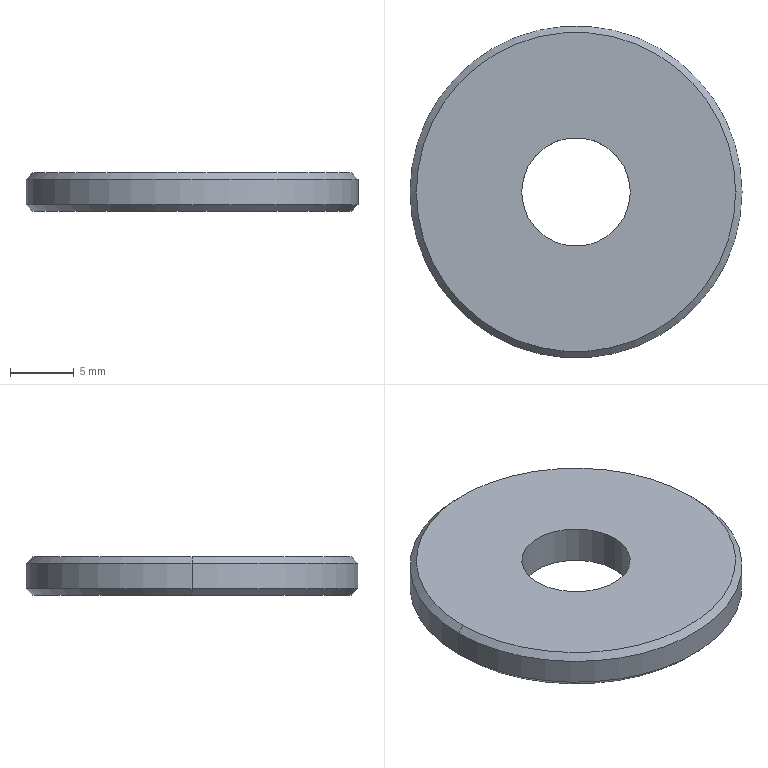Part | STEP file | 11-FG-SJ01711 | 1 solid | 10 faces | box 26 x 26 x 3 mm | volume 1402 mm3 | cone 4 | cylinder 4 | plane 2 | commonest cylinder face diameters 8.5 x2 26 x2
STEP:
#1=CARTESIAN_POINT('',(12.5,0.,3.));
#2=VERTEX_POINT('',#1);
#3=CARTESIAN_POINT('',(-12.5,0.,3.));
#4=VERTEX_POINT('',#3);
#5=CARTESIAN_POINT('',(0.,0.,3.));
#6=DIRECTION('',(0.,0.,1.));
#7=DIRECTION('',(1.,0.,0.));
#8=AXIS2_PLACEMENT_3D('',#5,#6,#7);
#9=CIRCLE('',#8,12.5);
#10=EDGE_CURVE('',#2,#4,#9,.T.);
#11=ORIENTED_EDGE('',*,*,#10,.F.);
#12=CARTESIAN_POINT('',(13.,0.,2.5));
#13=VERTEX_POINT('',#12);
#14=CARTESIAN_POINT('',(12.5,0.,3.));
#15=DIRECTION('',(0.7071,0.,-0.7071));
#16=VECTOR('',#15,1000.);
#17=LINE('',#14,#16);
#18=EDGE_CURVE('',#2,#13,#17,.T.);
#19=ORIENTED_EDGE('',*,*,#18,.T.);
#20=CARTESIAN_POINT('',(-13.,0.,2.5));
#21=VERTEX_POINT('',#20);
#22=CARTESIAN_POINT('',(0.,0.,2.5));
#23=DIRECTION('',(0.,0.,-1.));
#24=DIRECTION('',(1.,0.,0.));
#25=AXIS2_PLACEMENT_3D('',#22,#23,#24);
#26=CIRCLE('',#25,13.);
#27=EDGE_CURVE('',#21,#13,#26,.T.);
#28=ORIENTED_EDGE('',*,*,#27,.F.);
#29=CARTESIAN_POINT('',(-12.5,0.,3.));
#30=DIRECTION('',(-0.7071,0.,-0.7071));
#31=VECTOR('',#30,1000.);
#32=LINE('',#29,#31);
#33=EDGE_CURVE('',#4,#21,#32,.T.);
#34=ORIENTED_EDGE('',*,*,#33,.F.);
#35=EDGE_LOOP('',(#11,#19,#28,#34));
#36=FACE_OUTER_BOUND('',#35,.T.);
#37=CARTESIAN_POINT('',(0.,0.,3.));
#38=DIRECTION('',(0.,0.,-1.));
#39=DIRECTION('',(-1.,0.,0.));
#40=AXIS2_PLACEMENT_3D('',#37,#38,#39);
#41=CONICAL_SURFACE('',#40,12.5,0.7854);
#42=ADVANCED_FACE('',(#36),#41,.T.);
#43=CARTESIAN_POINT('',(-12.5,0.,0.));
#44=VERTEX_POINT('',#43);
#45=CARTESIAN_POINT('',(12.5,0.,0.));
#46=VERTEX_POINT('',#45);
#47=CARTESIAN_POINT('',(0.,0.,0.));
#48=DIRECTION('',(0.,0.,-1.));
#49=DIRECTION('',(1.,0.,0.));
#50=AXIS2_PLACEMENT_3D('',#47,#48,#49);
#51=CIRCLE('',#50,12.5);
#52=EDGE_CURVE('',#44,#46,#51,.T.);
#53=ORIENTED_EDGE('',*,*,#52,.F.);
#54=CARTESIAN_POINT('',(-13.,0.,0.5));
#55=VERTEX_POINT('',#54);
#56=CARTESIAN_POINT('',(-13.,0.,0.5));
#57=DIRECTION('',(-0.7071,0.,0.7071));
#58=VECTOR('',#57,1000.);
#59=LINE('',#56,#58);
#60=EDGE_CURVE('',#44,#55,#59,.T.);
#61=ORIENTED_EDGE('',*,*,#60,.T.);
#62=CARTESIAN_POINT('',(13.,0.,0.5));
#63=VERTEX_POINT('',#62);
#64=CARTESIAN_POINT('',(0.,0.,0.5));
#65=DIRECTION('',(0.,0.,1.));
#66=DIRECTION('',(1.,0.,0.));
#67=AXIS2_PLACEMENT_3D('',#64,#65,#66);
#68=CIRCLE('',#67,13.);
#69=EDGE_CURVE('',#63,#55,#68,.T.);
#70=ORIENTED_EDGE('',*,*,#69,.F.);
#71=CARTESIAN_POINT('',(13.,0.,0.5));
#72=DIRECTION('',(0.7071,0.,0.7071));
#73=VECTOR('',#72,1000.);
#74=LINE('',#71,#73);
#75=EDGE_CURVE('',#46,#63,#74,.T.);
#76=ORIENTED_EDGE('',*,*,#75,.F.);
#77=EDGE_LOOP('',(#53,#61,#70,#76));
#78=FACE_OUTER_BOUND('',#77,.T.);
#79=CARTESIAN_POINT('',(0.,0.,0.5));
#80=DIRECTION('',(0.,0.,1.));
#81=DIRECTION('',(1.,0.,0.));
#82=AXIS2_PLACEMENT_3D('',#79,#80,#81);
#83=CONICAL_SURFACE('',#82,13.,0.7854);
#84=ADVANCED_FACE('',(#78),#83,.T.);
#85=CARTESIAN_POINT('',(-4.25,0.,3.));
#86=VERTEX_POINT('',#85);
#87=CARTESIAN_POINT('',(4.25,0.,3.));
#88=VERTEX_POINT('',#87);
#89=CARTESIAN_POINT('',(0.,0.,3.));
#90=DIRECTION('',(0.,0.,1.));
#91=DIRECTION('',(1.,0.,0.));
#92=AXIS2_PLACEMENT_3D('',#89,#90,#91);
#93=CIRCLE('',#92,4.25);
#94=EDGE_CURVE('',#86,#88,#93,.T.);
#95=ORIENTED_EDGE('',*,*,#94,.T.);
#96=CARTESIAN_POINT('',(4.25,0.,0.));
#97=VERTEX_POINT('',#96);
#98=CARTESIAN_POINT('',(4.25,0.,3.));
#99=DIRECTION('',(0.,0.,-1.));
#100=VECTOR('',#99,1000.);
#101=LINE('',#98,#100);
#102=EDGE_CURVE('',#88,#97,#101,.T.);
#103=ORIENTED_EDGE('',*,*,#102,.T.);
#104=CARTESIAN_POINT('',(-4.25,0.,0.));
#105=VERTEX_POINT('',#104);
#106=CARTESIAN_POINT('',(0.,0.,0.));
#107=DIRECTION('',(0.,0.,1.));
#108=DIRECTION('',(1.,0.,0.));
#109=AXIS2_PLACEMENT_3D('',#106,#107,#108);
#110=CIRCLE('',#109,4.25);
#111=EDGE_CURVE('',#105,#97,#110,.T.);
#112=ORIENTED_EDGE('',*,*,#111,.F.);
#113=CARTESIAN_POINT('',(-4.25,0.,3.));
#114=DIRECTION('',(0.,0.,-1.));
#115=VECTOR('',#114,1000.);
#116=LINE('',#113,#115);
#117=EDGE_CURVE('',#86,#105,#116,.T.);
#118=ORIENTED_EDGE('',*,*,#117,.F.);
#119=EDGE_LOOP('',(#95,#103,#112,#118));
#120=FACE_OUTER_BOUND('',#119,.T.);
#121=CARTESIAN_POINT('',(0.,0.,3.));
#122=DIRECTION('',(0.,0.,-1.));
#123=DIRECTION('',(-1.,0.,0.));
#124=AXIS2_PLACEMENT_3D('',#121,#122,#123);
#125=CYLINDRICAL_SURFACE('',#124,4.25);
#126=ADVANCED_FACE('',(#120),#125,.F.);
#127=ORIENTED_EDGE('',*,*,#27,.T.);
#128=CARTESIAN_POINT('',(13.,0.,3.));
#129=DIRECTION('',(0.,0.,-1.));
#130=VECTOR('',#129,1000.);
#131=LINE('',#128,#130);
#132=EDGE_CURVE('',#13,#63,#131,.T.);
#133=ORIENTED_EDGE('',*,*,#132,.T.);
#134=ORIENTED_EDGE('',*,*,#69,.T.);
#135=CARTESIAN_POINT('',(-13.,0.,3.));
#136=DIRECTION('',(0.,0.,-1.));
#137=VECTOR('',#136,1000.);
#138=LINE('',#135,#137);
#139=EDGE_CURVE('',#21,#55,#138,.T.);
#140=ORIENTED_EDGE('',*,*,#139,.F.);
#141=EDGE_LOOP('',(#127,#133,#134,#140));
#142=FACE_OUTER_BOUND('',#141,.T.);
#143=CARTESIAN_POINT('',(0.,0.,3.));
#144=DIRECTION('',(0.,0.,-1.));
#145=DIRECTION('',(-1.,0.,0.));
#146=AXIS2_PLACEMENT_3D('',#143,#144,#145);
#147=CYLINDRICAL_SURFACE('',#146,13.);
#148=ADVANCED_FACE('',(#142),#147,.T.);
#149=CARTESIAN_POINT('',(0.,0.,3.));
#150=DIRECTION('',(0.,0.,1.));
#151=DIRECTION('',(1.,0.,0.));
#152=AXIS2_PLACEMENT_3D('',#149,#150,#151);
#153=CIRCLE('',#152,12.5);
#154=EDGE_CURVE('',#4,#2,#153,.T.);
#155=ORIENTED_EDGE('',*,*,#154,.T.);
#156=ORIENTED_EDGE('',*,*,#10,.T.);
#157=EDGE_LOOP('',(#155,#156));
#158=FACE_OUTER_BOUND('',#157,.T.);
#159=ORIENTED_EDGE('',*,*,#94,.F.);
#160=CARTESIAN_POINT('',(0.,0.,3.));
#161=DIRECTION('',(0.,0.,1.));
#162=DIRECTION('',(1.,0.,0.));
#163=AXIS2_PLACEMENT_3D('',#160,#161,#162);
#164=CIRCLE('',#163,4.25);
#165=EDGE_CURVE('',#88,#86,#164,.T.);
#166=ORIENTED_EDGE('',*,*,#165,.F.);
#167=EDGE_LOOP('',(#159,#166));
#168=FACE_BOUND('',#167,.T.);
#169=CARTESIAN_POINT('',(0.,0.,3.));
#170=DIRECTION('',(0.,0.,1.));
#171=DIRECTION('',(1.,0.,0.));
#172=AXIS2_PLACEMENT_3D('',#169,#170,#171);
#173=PLANE('',#172);
#174=ADVANCED_FACE('',(#158,#168),#173,.T.);
#175=CARTESIAN_POINT('',(0.,0.,0.));
#176=DIRECTION('',(0.,0.,-1.));
#177=DIRECTION('',(1.,0.,0.));
#178=AXIS2_PLACEMENT_3D('',#175,#176,#177);
#179=CIRCLE('',#178,12.5);
#180=EDGE_CURVE('',#46,#44,#179,.T.);
#181=ORIENTED_EDGE('',*,*,#180,.T.);
#182=ORIENTED_EDGE('',*,*,#52,.T.);
#183=EDGE_LOOP('',(#181,#182));
#184=FACE_OUTER_BOUND('',#183,.T.);
#185=ORIENTED_EDGE('',*,*,#111,.T.);
#186=CARTESIAN_POINT('',(0.,0.,0.));
#187=DIRECTION('',(0.,0.,1.));
#188=DIRECTION('',(1.,0.,0.));
#189=AXIS2_PLACEMENT_3D('',#186,#187,#188);
#190=CIRCLE('',#189,4.25);
#191=EDGE_CURVE('',#97,#105,#190,.T.);
#192=ORIENTED_EDGE('',*,*,#191,.T.);
#193=EDGE_LOOP('',(#185,#192));
#194=FACE_BOUND('',#193,.T.);
#195=CARTESIAN_POINT('',(0.,0.,0.));
#196=DIRECTION('',(0.,0.,1.));
#197=DIRECTION('',(1.,0.,0.));
#198=AXIS2_PLACEMENT_3D('',#195,#196,#197);
#199=PLANE('',#198);
#200=ADVANCED_FACE('',(#184,#194),#199,.F.);
#201=ORIENTED_EDGE('',*,*,#132,.F.);
#202=CARTESIAN_POINT('',(0.,0.,2.5));
#203=DIRECTION('',(0.,0.,-1.));
#204=DIRECTION('',(1.,0.,0.));
#205=AXIS2_PLACEMENT_3D('',#202,#203,#204);
#206=CIRCLE('',#205,13.);
#207=EDGE_CURVE('',#13,#21,#206,.T.);
#208=ORIENTED_EDGE('',*,*,#207,.T.);
#209=ORIENTED_EDGE('',*,*,#139,.T.);
#210=CARTESIAN_POINT('',(0.,0.,0.5));
#211=DIRECTION('',(0.,0.,1.));
#212=DIRECTION('',(1.,0.,0.));
#213=AXIS2_PLACEMENT_3D('',#210,#211,#212);
#214=CIRCLE('',#213,13.);
#215=EDGE_CURVE('',#55,#63,#214,.T.);
#216=ORIENTED_EDGE('',*,*,#215,.T.);
#217=EDGE_LOOP('',(#201,#208,#209,#216));
#218=FACE_OUTER_BOUND('',#217,.T.);
#219=CARTESIAN_POINT('',(0.,0.,3.));
#220=DIRECTION('',(0.,0.,-1.));
#221=DIRECTION('',(-1.,0.,0.));
#222=AXIS2_PLACEMENT_3D('',#219,#220,#221);
#223=CYLINDRICAL_SURFACE('',#222,13.);
#224=ADVANCED_FACE('',(#218),#223,.T.);
#225=ORIENTED_EDGE('',*,*,#102,.F.);
#226=ORIENTED_EDGE('',*,*,#165,.T.);
#227=ORIENTED_EDGE('',*,*,#117,.T.);
#228=ORIENTED_EDGE('',*,*,#191,.F.);
#229=EDGE_LOOP('',(#225,#226,#227,#228));
#230=FACE_OUTER_BOUND('',#229,.T.);
#231=CARTESIAN_POINT('',(0.,0.,3.));
#232=DIRECTION('',(0.,0.,-1.));
#233=DIRECTION('',(-1.,0.,0.));
#234=AXIS2_PLACEMENT_3D('',#231,#232,#233);
#235=CYLINDRICAL_SURFACE('',#234,4.25);
#236=ADVANCED_FACE('',(#230),#235,.F.);
#237=ORIENTED_EDGE('',*,*,#60,.F.);
#238=ORIENTED_EDGE('',*,*,#180,.F.);
#239=ORIENTED_EDGE('',*,*,#75,.T.);
#240=ORIENTED_EDGE('',*,*,#215,.F.);
#241=EDGE_LOOP('',(#237,#238,#239,#240));
#242=FACE_OUTER_BOUND('',#241,.T.);
#243=CARTESIAN_POINT('',(0.,0.,0.5));
#244=DIRECTION('',(0.,0.,1.));
#245=DIRECTION('',(1.,0.,0.));
#246=AXIS2_PLACEMENT_3D('',#243,#244,#245);
#247=CONICAL_SURFACE('',#246,13.,0.7854);
#248=ADVANCED_FACE('',(#242),#247,.T.);
#249=ORIENTED_EDGE('',*,*,#18,.F.);
#250=ORIENTED_EDGE('',*,*,#154,.F.);
#251=ORIENTED_EDGE('',*,*,#33,.T.);
#252=ORIENTED_EDGE('',*,*,#207,.F.);
#253=EDGE_LOOP('',(#249,#250,#251,#252));
#254=FACE_OUTER_BOUND('',#253,.T.);
#255=CARTESIAN_POINT('',(0.,0.,3.));
#256=DIRECTION('',(0.,0.,-1.));
#257=DIRECTION('',(-1.,0.,0.));
#258=AXIS2_PLACEMENT_3D('',#255,#256,#257);
#259=CONICAL_SURFACE('',#258,12.5,0.7854);
#260=ADVANCED_FACE('',(#254),#259,.T.);
#261=CLOSED_SHELL('',(#42,#84,#126,#148,#174,#200,#224,#236,#248,#260));
#262=MANIFOLD_SOLID_BREP('',#261);
#263=CARTESIAN_POINT('',(0.,0.,0.));
#264=DIRECTION('',(0.,0.,1.));
#265=DIRECTION('',(1.,0.,0.));
#266=AXIS2_PLACEMENT_3D('',#263,#264,#265);
#267=(LENGTH_UNIT()NAMED_UNIT(*)SI_UNIT(.MILLI.,.METRE.));
#268=UNCERTAINTY_MEASURE_WITH_UNIT(LENGTH_MEASURE(0.00001),#267,'','');
#269=(NAMED_UNIT(*)PLANE_ANGLE_UNIT()SI_UNIT($,.RADIAN.));
#270=(NAMED_UNIT(*)SI_UNIT($,.STERADIAN.)SOLID_ANGLE_UNIT());
#271=(GEOMETRIC_REPRESENTATION_CONTEXT(3)GLOBAL_UNCERTAINTY_ASSIGNED_CONTEXT((#268))GLOBAL_UNIT_ASSIGNED_CONTEXT((#267,#269,#270))REPRESENTATION_CONTEXT('',''));
#272=ADVANCED_BREP_SHAPE_REPRESENTATION('',(#262,#266),#271);